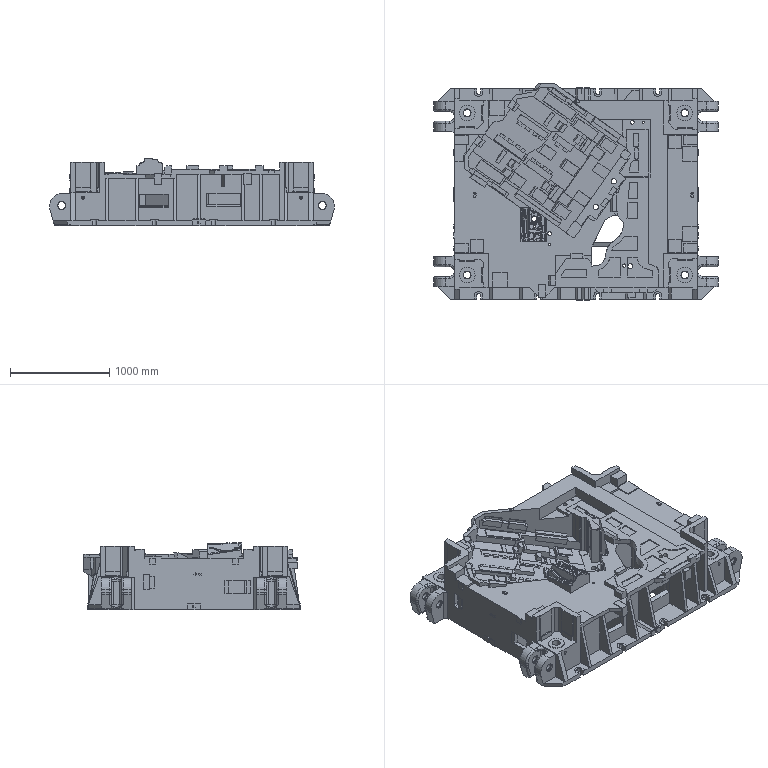Part | NX | features solid 2 | 1 solid | 2483 faces | box 2860 x 2180 x 681.51 mm | volume 869453208 mm3 | plane 1854 | cylinder 308 | spline 293 | torus 28 | commonest cylinder face diameters 40 x59 80 x56 83 x48 60 x32 30 x20 100 x20